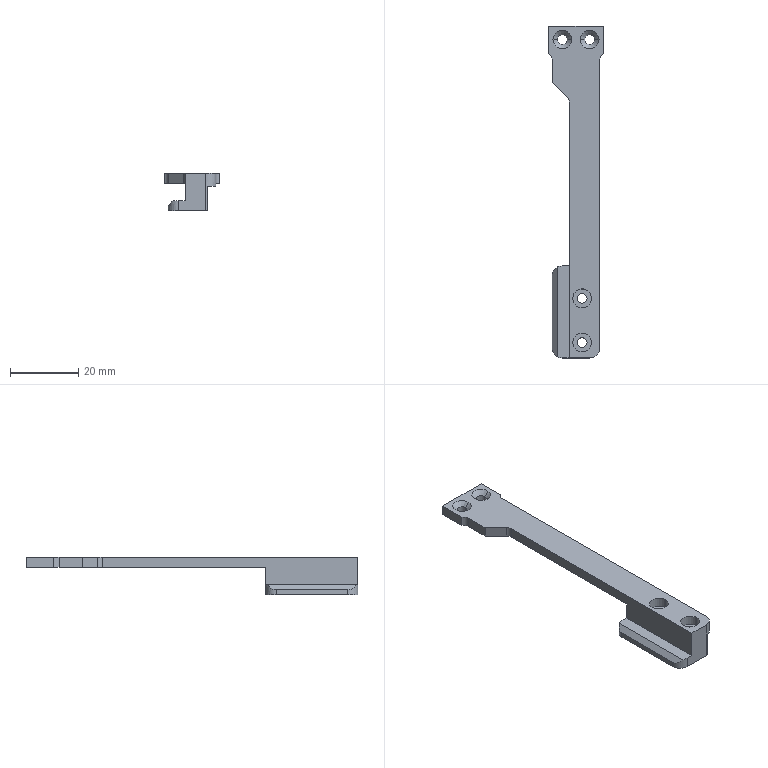NC program | NX | posted with a generic post | part box 16 x 97.4 x 11 mm
Whole program, first 1466 of 1616 lines:
N10 G17 G21 G94 G90
(ADAPTIVE_MILLING_1 , TOOL : D8-25-D8-60-3T-ROUGH)
N12 T02 M6
N14 G54
N16 G17 G0 G90 X-46.305 Y19.064 S6500 M3
N18 G43 Z20. H2
N20 Z-4.9
N22 G94 G1 X-46.303 Y18.914 Z-5.837 F3000.
N24 X-46.3 Y18.764 Z-6.208
N26 X-46.298 Y18.614 Z-6.48
N28 X-46.295 Y18.464 Z-6.7
N30 X-46.293 Y18.314 Z-6.884
N32 X-46.29 Y18.164 Z-7.042
N34 X-46.288 Y18.014 Z-7.18
N36 X-46.286 Y17.864 Z-7.3
N38 X-46.283 Y17.714 Z-7.405
N40 X-46.281 Y17.564 Z-7.498
N42 X-46.278 Y17.414 Z-7.579
N44 X-46.276 Y17.264 Z-7.65
N46 X-46.273 Y17.114 Z-7.71
N48 X-46.271 Y16.964 Z-7.762
N50 X-46.268 Y16.814 Z-7.805
N52 X-46.266 Y16.664 Z-7.839
N54 X-46.263 Y16.514 Z-7.866
N56 X-46.261 Y16.364 Z-7.885
N58 X-46.258 Y16.214 Z-7.896
N60 X-46.256 Y16.064 Z-7.9
N62 X-46.235 Y14.789
N64 G3 X-45.716 Y14.048 R0.809
N66 X-44.438 Y13.739 R5.226
N68 X-41.665 Y13.553 R27.344
N70 X-35.265 Y13.499 R256.654
N72 G1 X49.64
N74 X50.281 Y13.501
N76 X50.921 Y13.487
N78 G2 X53.296 Y12.469 R4.266
N80 X54.935 Y10.214 R6.112
N82 X55.663 Y7.571 R10.548
N84 X55.934 Y4.208 R28.629
N86 X55.996 Y-2.229 R222.094
N88 G1 X55.993 Y-8.303
N90 G2 X55.042 Y-10.705 R4.206
N92 X52.82 Y-12.386 R6.008
N94 X50.123 Y-13.155 R10.335
N96 X46.7 Y-13.435 R28.276
N98 X40.263 Y-13.497 R221.026
N100 G1 X-49.835 Y-13.498
N102 X-50.96 Y-13.483
N104 G2 X-53.325 Y-12.441 R4.293
N106 X-54.923 Y-10.232 R6.094
N108 X-55.667 Y-7.528 R10.64
N110 X-55.933 Y-4.228 R28.613
N112 X-55.996 Y2.209 R217.689
N114 G1 X-56. Y5.266
N116 X-55.992 Y8.324
N118 G2 X-55.066 Y10.671 R4.211
N120 X-52.856 Y12.367 R5.966
N122 X-50.224 Y13.137 R10.16
N124 X-47.3 Y13.377 R16.967
N126 G1 X-46.006 Y13.318
N128 X-44.713 Y13.227
N130 G3 X-38.795 Y13.02 R97.929
N132 G1 X-35.624 Y13.003
N134 X-32.453 Y12.999
N136 X48.734
N138 G2 X52.851 Y11.189 R5.658
N140 X54.443 Y8.596 R7.718
N142 X55.173 Y5.564 R13.413
N144 X55.442 Y1.637 R37.942
N146 X55.492 Y-6.425 R312.321
N148 X53.773 Y-10.266 R5.637
N150 X51.201 Y-11.901 R7.615
N152 X48.177 Y-12.657 R13.076
N154 X44.376 Y-12.936 R35.501
N156 X37.752 Y-12.997 R250.241
N158 G1 X35.002 Y-12.998
N160 X-48.853 Y-12.996
N162 G2 X-52.846 Y-11.19 R5.661
N164 X-54.445 Y-8.582 R7.749
N166 X-55.173 Y-5.551 R13.49
N168 X-55.438 Y-1.749 R37.037
N170 X-55.496 Y5.126 R274.031
N172 G1 X-55.5 Y5.875
N174 X-55.481 Y6.625
N176 G2 X-53.801 Y10.236 R5.633
N178 X-51.157 Y11.916 R7.618
N180 X-47.871 Y12.628 R11.221
N182 X-44.748 Y12.667 R30.947
N184 G3 X-33.138 Y12.501 R329.166
N186 G1 X-29.641 Y12.499
N188 X46.922
N190 G2 X49.208 Y12.216 R7.846
N192 X52.557 Y9.903 R6.635
N194 X54.044 Y7.031 R9.19
N196 X54.713 Y3.726 R16.717
N198 X54.947 Y-0.328 R47.28
N200 X54.983 Y-4.953 R131.72
N202 X52.578 Y-9.913 R6.579
N204 X49.608 Y-11.519 R9.017
N206 X46.309 Y-12.204 R16.357
N208 X42.318 Y-12.444 R45.46
N210 X34.755 Y-12.497 R345.421
N212 G1 X-46.132 Y-12.498
N214 X-47.819 Y-12.466
N216 G2 X-52.408 Y-10.084 R6.561
N218 X-54.009 Y-7.135 R8.99
N220 X-54.706 Y-3.774 R16.39
N222 X-54.945 Y0.28 R46.219
N224 G1 X-54.981 Y2.561
N226 X-54.986 Y4.842
N228 G2 X-54.068 Y8.178 R6.681
N230 X-51.185 Y10.832 R7.188
N232 X-48.101 Y11.819 R10.315
N234 X-44.864 Y12.076 R22.321
N236 G1 X-43.864 Y12.085
N238 X-27.664
N240 G3 X-22.382 Y12.005 R137.915
N242 G1 X-18.516 Y11.999
N244 X45.309
N246 G2 X47.427 Y11.86 R12.199
N248 X51.964 Y9.081 R7.185
N250 X53.51 Y6.019 R9.94
N252 X54.187 Y2.652 R17.79
N254 X54.442 Y-1.651 R48.718
N256 X54.447 Y-3.963 R31.467
N258 X53.495 Y-7.299 R7.389
N260 X50.775 Y-10.007 R7.645
N262 X47.652 Y-11.253 R11.295
N264 X44.071 Y-11.792 R22.406
N266 X39.45 Y-11.969 R72.829
N268 G1 X35.669 Y-11.994
N270 X31.888 Y-11.997
N272 X-44.603
N274 G2 X-46.602 Y-11.959 R27.447
N276 X-50.282 Y-10.698 R7.293
N278 X-52.732 Y-7.883 R7.956
N280 X-53.869 Y-4.648 R12.187
N282 X-54.34 Y-0.868 R26.01
N284 X-54.46 Y3.629 R66.215
N286 X-53.891 Y6.494 R7.865
N288 X-51.028 Y9.807 R7.178
N290 X-47.967 Y11.035 R10.032
N292 X-44.749 Y11.463 R19.383
N294 X-40.001 Y11.574 R90.869
N296 G1 X-33.376 Y11.584
N298 X-30.43 Y11.587
N300 X-27.484 Y11.579
N302 G3 X-18.952 Y11.501 R345.09
N304 G1 X-16.204 Y11.5
N306 X43.871
N308 G2 X46.117 Y11.392 R17.117
N310 X51.451 Y8.231 R7.693
N312 X53.002 Y5.033 R10.645
N314 X53.682 Y1.541 R19.181
N316 X53.907 Y-2.513 R36.968
N318 X53.443 Y-5.337 R8.745
N320 X50.631 Y-9.009 R7.665
N322 X47.419 Y-10.533 R10.754
N324 X43.861 Y-11.201 R19.666
N326 X39.494 Y-11.444 R54.318
N328 X31.557 Y-11.497 R385.627
N330 G1 X30.182
N332 X-43.041
N334 G2 X-45.415 Y-11.459 R38.148
N336 X-48.492 Y-10.706 R8.396
N338 X-51.113 Y-8.66 R7.694
N340 G1 X-51.369 Y-8.359
N342 X-51.597 Y-8.036
N344 G2 X-53.07 Y-4.809 R11.035
N346 X-53.713 Y-1.246 R20.386
N348 X-53.906 Y2.56 R36.428
N350 X-53.423 Y5.38 R8.597
N352 X-51.336 Y8.39 R7.279
N354 X-50.295 Y9.478 R11.092
N356 G1 X-49.274 Y10.193
N358 X-48.144 Y10.719
N360 X-46.94 Y11.041
N362 X-45.7 Y11.15
N364 X-24.699
N366 G3 X-20.606 Y11.02 R66.565
N368 G1 X-17.374 Y11.003
N370 X-14.141 Y11.
N372 X42.559
N374 G2 X45.055 Y10.896 R21.521
N376 X48.627 Y9.662 R8.332
N378 X51.431 Y6.654 R8.583
N380 X52.72 Y3.274 R12.664
N382 X53.306 Y-1.682 R23.115
N384 X52.76 Y-4.804 R8.748
N386 X49.991 Y-8.364 R7.928
N388 X46.743 Y-9.949 R10.964
N390 X43.069 Y-10.67 R19.839
N392 X38.453 Y-10.939 R54.157
N394 X30.516 Y-10.996 R368.029
N396 G1 X-22.68 Y-10.997
N398 G3 X-23.46 Y-11.041 R3.21
N400 G1 X-24.701 Y-11.15
N402 X-45.701
N404 X-46.943 Y-11.041
N406 X-48.147 Y-10.718
N408 X-49.276 Y-10.191
N410 X-50.297 Y-9.476
N412 X-51.178 Y-8.595
N414 X-51.893 Y-7.574
N416 X-52.419 Y-6.444
N418 X-52.741 Y-5.24
N420 G2 X-53.283 Y0.049 R143.418
N422 X-53.035 Y3.961 R12.001
N424 G1 X-52.78 Y4.797
N426 X-52.741 Y5.243
N428 X-52.418 Y6.447
N430 X-51.891 Y7.576
N432 X-51.246 Y8.498
N434 G3 X-52.247 Y9.678 R0.8
N436 G1 X-52.451 Y9.545 Z-7.885
N438 X-52.641 Y9.393 Z-7.869
N440 X-53.503 Y8.717 Z-7.8
N442 X-54.402 Y8.012 F15000.
N444 G3 X-54.685 Y7.576 R0.808
N446 G1 X-55.007 Y6.299
N448 X-55.312 Y5.017
N450 G3 X-55.708 Y1.761 R18.608
N452 G1 X-55.863 Y-3.024
N454 G3 X-55.683 Y-3.556 R0.806
N456 G1 X-54.789 Y-4.653
N458 X-54.152 Y-5.426 Z-7.863 F3000.
N460 G3 X-53.641 Y-5.672 Z-7.9 R0.801
N462 X-52.78 Y-4.804 R0.8
N464 G1 X-52.85 Y-3.999
N466 Y4.001
N468 X-52.779 Y4.81
N470 G3 X-53.012 Y5.448 R0.802
N472 G1 X-53.247 Y5.681
N474 X-54.37 Y6.796 Z-7.8
N476 G2 X-54.689 Y7.369 R0.887 F15000.
N478 X-54.559 Y7.893 R0.807
N480 G1 X-52.913 Y10.362
N482 G2 X-51.228 Y11.971 R5.479
N484 X-49.816 Y12.657 R7.452
N486 X-47.934 Y13.222 R12.236
N488 X-45.983 Y13.437 R12.22
N490 X-42.036 Y13.56 R84.088
N492 G1 X-27.092 Y13.656
N494 G2 X-26.429 Y13.312 R0.802
N496 G1 X-26.31 Y13.14
N498 X-25.41 Y11.838 Z-7.9 F3000.
N500 X-25.254 Y11.611
N502 X-25.089 Y11.39
N504 G3 X-24.575 Y11.139 R0.806
N506 G1 X-23.457 Y11.041
N508 G3 X-20.1 Y10.593 R13.649
N510 X-11.516 Y10.5 R239.739
N512 G1 X41.684 Y10.499
N514 G2 X45.592 Y10.12 R15.22
N516 X51.095 Y5.539 R8.644
N518 X52.607 Y-1.982 R15.053
N520 X48.383 Y-8.371 R8.14
N522 X43.296 Y-10.009 R14.576
N524 X36.378 Y-10.458 R52.796
N526 X27.691 Y-10.496 R660.518
N528 G1 X-21.583 Y-10.498
N530 G3 X-22.256 Y-10.719 R1.464
N532 G1 X-23.403 Y-11.026
N534 G3 X-23.833 Y-11.316 R0.808
N536 G1 X-24.25 Y-11.865
N538 X-25.206 Y-13.126 Z-7.8
N540 G2 X-25.798 Y-13.534 R0.886 F15000.
N542 G1 X-25.92 Y-13.544
N544 X-46.688
N546 G2 X-49.702 Y-12.778 R6.536
N548 G1 X-50.044 Y-12.585
N550 X-50.377 Y-12.376
N552 X-52.02 Y-11.268
N554 G2 X-53.343 Y-9.871 R4.439
N556 X-54.449 Y-7.781 R20.2
N558 X-54.909 Y-6.279 R7.49
N560 X-55.563 Y-1.885 R46.393
N562 X-55.504 Y3.02 R19.609
N564 G1 X-55.31 Y4.44
N566 X-55.102 Y5.858
N568 G2 X-53.8 Y9.132 R9.034
N570 G1 X-53.443 Y9.685
N572 X-53.078 Y10.232
N574 G2 X-51.318 Y11.875 R6.623
N576 X-49.37 Y12.813 R9.364
N578 X-46.503 Y13.52 R16.251
N580 X-45.032 Y13.634 R12.935
N582 G1 X-24.694 Y13.979
N584 G2 X-23.899 Y13.352 R0.8
N586 G1 X-23.839 Y13.08
N588 X-23.497 Y11.535 Z-7.9 F3000.
N590 G3 X-22.914 Y10.895 R0.804
N592 G1 X-21.411 Y10.452
N594 G3 X-17.104 Y10.06 R24.39
N596 X-8.953 Y10. R461.545
N598 G1 X40.497 Y9.999
N600 G2 X44.537 Y9.671 R18.213
N602 X50.574 Y4.798 R8.931
N604 X51.9 Y-1.366 R12.155
N606 X47.893 Y-7.674 R8.103
N608 X42.598 Y-9.472 R14.422
N610 X35.37 Y-9.957 R52.872
N612 X26.12 Y-9.996 R677.713
N614 G1 X-19.96 Y-9.997
N616 G3 X-20.964 Y-10.097 R2.886
N618 G1 X-21.919 Y-10.562
N620 G3 X-22.345 Y-11.048 R0.803
N622 G1 X-22.467 Y-11.439
N624 X-22.941 Y-12.948 Z-7.8
N626 G2 X-23.202 Y-13.432 R0.972 F15000.
N628 X-23.699 Y-13.646 R0.807
N630 G1 X-27.811 Y-13.897
N632 X-31.924 Y-14.131
N634 G2 X-42.441 Y-13.875 R77.782
N636 G1 X-47.365 Y-13.42
N638 G2 X-49.982 Y-12.631 R7.102
N640 X-50.987 Y-12.013 R8.643
N642 G1 X-51.549 Y-11.611
N644 X-52.102 Y-11.197
N646 G2 X-53.85 Y-9.092 R7.418
N648 X-54.848 Y-6.533 R10.673
N650 X-55.5 Y-3.642 R39.775
N652 X-55.614 Y-1.681 R8.461
N654 G1 X-55.207 Y5.23
N656 G2 X-54.627 Y7.498 R6.215
N658 X-53.85 Y8.866 R8.818
N660 G1 X-52.812 Y10.347
N662 G2 X-52.046 Y11.203 R5.737
N664 G1 X-51.854 Y11.357
N666 X-51.656 Y11.502
N668 X-51.071 Y11.893
N670 X-50.478 Y12.274
N672 G2 X-48.149 Y13.179 R7.708
N674 X-45.216 Y13.504 R15.237
N676 G1 X-23.977 Y13.775
N678 G2 X-23.197 Y13.195 R0.8
N680 G1 X-23.146 Y13.013
N682 X-22.712 Y11.492 Z-7.9 F3000.
N684 X-22.652 Y11.279
N686 X-22.579 Y11.07
N688 G3 X-22.197 Y10.692 R0.807
N690 X-18.86 Y9.763 R8.541
N692 X-11.565 Y9.508 R77.946
N694 G1 X-6.953 Y9.501
N696 X39.497 Y9.499
N698 G2 X43.786 Y9.155 R19.531
N700 X50.097 Y3.988 R9.196
N702 X51.053 Y-1.474 R9.498
N704 X47.268 Y-7.053 R8.029
N706 X42.064 Y-8.91 R14.124
N708 X35.153 Y-9.44 R47.679
N710 X24.84 Y-9.496 R685.121
N712 G1 X-18.582 Y-9.498
N714 G3 X-20.271 Y-9.629 R7.598
N716 X-21.095 Y-10.171 R5.028
N718 X-21.435 Y-10.861 R0.801
N720 G1 X-21.262 Y-12.434 Z-7.8
N722 X-21.239 Y-12.644 F15000.
N724 X-21.227 Y-12.855
N726 G2 X-22.016 Y-13.61 R0.8
N728 G1 X-43.772 Y-13.861
N730 G2 X-48.086 Y-13.278 R14.904
N732 X-51.156 Y-11.714 R9.781
N734 G1 X-51.943 Y-11.118
N736 X-52.724 Y-10.514
N738 X-53.006 Y-10.276
N740 X-53.277 Y-10.024
N742 G2 X-53.71 Y-9.434 R2.98
N744 X-54.447 Y-7.93 R11.151
N746 X-55.146 Y-5.267 R14.703
N748 X-55.278 Y-3.798 R12.377
N750 G1 X-55.44 Y2.203
N752 G2 X-54.849 Y6.916 R15.719
N754 G1 X-54.675 Y7.533
N756 X-54.488 Y8.145
N758 G2 X-53.144 Y10.276 R5.71
N760 X-51.595 Y11.647 R11.819
N762 X-49.512 Y12.742 R7.979
N764 X-47.421 Y13.313 R11.302
N766 X-46.168 Y13.429 R10.126
N768 X-37.272 Y13.575 R312.239
N770 G1 X-25.967 Y13.581
N772 G2 X-24.11 Y13.493 R20.526
N774 G1 X-23.184 Y13.405
N776 G2 X-22.499 Y12.857 R0.801
N778 G1 X-22.007 Y11.353 Z-7.9 F3000.
N780 X-21.899 Y11.013
N782 X-21.775 Y10.678
N784 G3 X-21.404 Y10.322 R0.808
N786 X-20.449 Y9.841 R23.478
N788 X-16.974 Y9.204 R13.12
N790 X-9.382 Y9.006 R111.302
N792 G1 X-5.016 Y9.001
N794 X38.309 Y9.
N796 G2 X42.73 Y8.71 R23.559
N798 X50.265 Y0.302 R9.178
N800 X47.195 Y-6.022 R7.56
N802 X42.185 Y-8.213 R12.5
N804 X35.605 Y-8.9 R36.911
N806 X24.168 Y-8.996 R404.381
N808 G1 X-16.97
N810 G3 X-19.6 Y-9.151 R13.964
N812 X-20.105 Y-9.478 R1.054
N814 G1 X-20.464 Y-9.729
N816 G3 X-20.802 Y-10.446 R0.801
N818 G1 X-20.792 Y-10.58
N820 X-20.67 Y-12.158 Z-7.8
N822 G2 X-20.716 Y-12.675 R1.011 F15000.
N824 X-21.385 Y-13.168 R0.801
N826 G1 X-23.451 Y-13.352
N828 X-25.518 Y-13.522
N830 G2 X-30.253 Y-13.665 R61.669
N832 G1 X-45.584 Y-13.533
N834 G2 X-49.302 Y-12.883 R11.335
N836 X-51.182 Y-11.951 R9.638
N838 X-52.122 Y-11.298 R8.244
N840 X-52.988 Y-10.338 R4.901
N842 X-54.222 Y-8.319 R20.738
N844 X-54.773 Y-6.85 R7.392
N846 X-55.528 Y-3.478 R43.944
N848 X-55.673 Y-0.539 R11.383
N850 G1 X-55.204 Y5.261
N852 G2 X-54.264 Y8.362 R7.66
N854 X-49.785 Y12.663 R10.114
N856 X-47.384 Y13.351 R7.726
N858 X-44.43 Y13.526 R25.996
N860 G1 X-21.943 Y13.559
N862 G2 X-21.147 Y12.666 R0.8
N864 G1 X-21.175 Y12.426
N866 X-21.359 Y10.854 Z-7.9 F3000.
N868 G3 X-21.022 Y10.12 R0.801
N870 X-18.496 Y9.049 R5.612
N872 X-13.225 Y8.574 R32.298
N874 X-3.329 Y8.501 R443.883
N876 G1 X37.246 Y8.5
N878 G2 X41.857 Y8.227 R26.64
N880 X48.574 Y3.376 R9.125
N882 X47.062 Y-4.888 R7.016
N884 X42.272 Y-7.472 R11.027
N886 X36.157 Y-8.335 R28.801
N888 X24.659 Y-8.495 R242.942
N890 G1 X-15.351
N892 G3 X-18.78 Y-8.639 R23.511
N894 X-19.545 Y-8.918 R1.61
N896 G1 X-19.987 Y-9.36
N898 G3 X-20.22 Y-9.884 R0.806
N900 G1 X-20.248 Y-10.42
N902 X-20.33 Y-12.001 Z-7.8
N904 G2 X-20.908 Y-12.799 R0.808 F15000.
N906 G1 X-22.238 Y-13.179
N908 G2 X-23.793 Y-13.427 R9.587
N910 G1 X-27.834 Y-13.734
N912 X-31.876 Y-14.023
N914 G2 X-42.521 Y-13.849 R71.443
N916 G1 X-47.446 Y-13.399
N918 G2 X-49.685 Y-12.729 R5.967
N920 X-51.017 Y-11.89 R8.858
N922 G1 X-51.801 Y-11.292
N924 X-52.577 Y-10.684
N926 X-52.857 Y-10.443
N928 X-53.125 Y-10.188
N930 G2 X-53.552 Y-9.593 R3.011
N932 X-54.717 Y-6.993 R14.622
N934 X-55.05 Y-5.459 R8.844
N936 G1 X-55.28 Y-3.622
N938 X-55.494 Y-1.783
N940 G2 X-55.406 Y3.37 R23.638
N942 G1 X-55.284 Y4.351
N944 X-55.145 Y5.329
N946 G2 X-54.436 Y7.669 R10.28
N948 X-53.492 Y9.507 R11.89
N950 X-51.925 Y11.248 R6.735
N952 X-49.848 Y12.557 R13.665
N954 X-48.735 Y13.088 R10.021
N956 X-48.02 Y13.254 R3.368
N958 X-44.829 Y13.526 R36.806
N960 G1 X-44.09 Y13.54
N962 X-26.79 Y13.631
N964 G2 X-23.213 Y13.42 R28.16
N966 G1 X-21.431 Y13.2
N968 G2 X-20.731 Y12.356 R0.8
N970 G1 X-20.739 Y12.222
N972 X-20.838 Y10.643 Z-7.9 F3000.
N974 G3 X-20.82 Y10.197 R1.186
N976 X-20.51 Y9.761 R0.807
N978 X-17.799 Y8.588 R6.045
N980 X-12.344 Y8.082 R33.074
N982 X-2.828 Y8.001 R398.643
N984 G1 X36.247 Y8.
N986 G2 X41.046 Y7.736 R29.411
N988 X46.582 Y4.803 R9.282
N990 X46.574 Y-3.923 R6.511
N992 X42.122 Y-6.742 R9.967
N994 X36.289 Y-7.767 R23.955
N996 X27.043 Y-7.99 R143.085
N998 G1 X22.231 Y-7.995
N1000 X-14.719 Y-7.996
N1002 G3 X-18.294 Y-8.179 R22.526
N1004 X-19.2 Y-8.563 R1.558
N1006 X-19.302 Y-9.265 R0.802
N1008 G1 X-19.252 Y-9.419
N1010 X-18.762 Y-10.924 Z-7.8
N1012 G2 X-18.659 Y-11.391 R1.333 F15000.
N1014 X-19.2 Y-12.123 R0.801
N1016 G1 X-20.366 Y-12.525
N1018 X-21.536 Y-12.913
N1020 G2 X-24.914 Y-13.457 R12.999
N1022 X-31.832 Y-13.577 R267.609
N1024 G1 X-45.787 Y-13.624
N1026 G2 X-49.391 Y-12.935 R9.6
N1028 X-51.343 Y-11.904 R8.067
N1030 X-52.525 Y-10.84 R9.768
N1032 X-53.98 Y-8.867 R8.328
N1034 X-54.835 Y-6.774 R9.887
N1036 X-55.044 Y-5.614 R7.91
N1038 G1 X-55.636 Y0.287
N1040 G2 X-55.471 Y4.2 R13.827
N1042 X-53.986 Y8.664 R14.774
N1044 X-52.718 Y10.415 R9.474
N1046 X-51.42 Y11.617 R9.301
N1048 X-50.417 Y12.236 R7.368
N1050 X-48.819 Y12.948 R11.429
N1052 X-47.192 Y13.344 R9.224
N1054 X-44.247 Y13.575 R21.928
N1056 G1 X-25.104 Y13.776
N1058 G2 X-22.361 Y13.353 R8.536
N1060 G1 X-21.025 Y12.915
N1062 G2 X-20.475 Y12.205 R0.801
N1064 G1 X-20.468 Y12.092
N1066 X-20.369 Y10.513 Z-7.9 F3000.
N1068 X-20.351 Y10.195
N1070 X-20.32 Y9.877
N1072 G3 X-20.103 Y9.476 R0.814
N1074 X-18.296 Y8.424 R4.02
N1076 X-13.944 Y7.71 R18.688
N1078 X-5.26 Y7.505 R138.606
N1080 G1 X-1.141 Y7.501
N1082 X35.184
N1084 G2 X40.049 Y7.277 R34.755
N1086 X44.892 Y5.254 R9.571
N1088 X45.883 Y-2.999 R5.985
N1090 X41.736 Y-6.038 R9.034
N1092 X36.059 Y-7.211 R20.853
N1094 X27.253 Y-7.486 R112.741
N1096 G1 X21.066 Y-7.495
N1098 X-13.841 Y-7.496
N1100 G3 X-17.656 Y-7.683 R26.495
N1102 X-18.851 Y-8.105 R2.625
N1104 X-19.224 Y-8.597 R6.533
N1106 G1 X-19.577 Y-8.95
N1108 G3 X-19.774 Y-9.76 R0.801
N1110 G1 X-19.128 Y-11.204 Z-7.8
N1112 G2 X-18.971 Y-11.65 R1.452 F15000.
N1114 X-19.577 Y-12.511 R0.8
N1116 G1 X-20.856 Y-12.824
N1118 X-22.137 Y-13.124
N1120 G2 X-25.39 Y-13.546 R21.019
N1122 G1 X-37.244 Y-14.145
N1124 G2 X-45.107 Y-13.758 R39.527
N1126 G1 X-46.537 Y-13.546
N1128 X-47.966 Y-13.319
N1130 G2 X-50.995 Y-12.174 R9.363
N1132 X-52.654 Y-10.753 R7.079
N1134 X-53.675 Y-9.427 R10.481
N1136 X-54.995 Y-6.151 R10.707
N1138 X-55.16 Y-4.982 R9.43
N1140 G1 X-55.598 Y0.936
N1142 G2 X-55.346 Y4.846 R14.219
N1144 G1 X-55.058 Y6.199
N1146 G2 X-53.518 Y9.362 R9.128
N1148 G1 X-53.106 Y9.916
N1150 X-52.683 Y10.462
N1152 G2 X-50.894 Y11.985 R7.54
N1154 X-47.24 Y13.408 R10.85
N1156 X-46.066 Y13.536 R9.123
N1158 G1 X-26.315 Y14.308
N1160 G2 X-22.578 Y13.54 R7.967
N1162 G1 X-20.804 Y12.694
N1164 G2 X-20.351 Y12.042 R0.802
N1166 G1 X-20.188 Y10.468 Z-7.9 F3000.
N1168 X-20.112 Y9.738
N1170 G3 X-19.882 Y9.255 R0.807
N1172 X-17.794 Y7.979 R4.417
N1174 X-13.251 Y7.224 R19.503
N1176 X-3.699 Y7.004 R147.219
N1178 G1 X-0.953 Y7.002
N1180 X34.247 Y7.001
N1182 G2 X39.3 Y6.779 R37.483
N1184 X43.487 Y5.248 R9.4
N1186 X45.02 Y-2.037 R5.47
N1188 X41.252 Y-5.304 R8.085
N1190 X35.936 Y-6.625 R17.55
N1192 X27.822 Y-6.975 R82.824
N1194 G1 X20.259 Y-6.994
N1196 X-12.719 Y-6.995
N1198 G3 X-17.054 Y-7.19 R31.774
N1200 X-18.526 Y-7.661 R3.673
N1202 X-18.982 Y-8.252 R3.018
N1204 X-19.112 Y-8.868 R0.804
N1206 G1 X-19.02 Y-9.327
N1208 X-18.711 Y-10.879 Z-7.8
N1210 G2 X-18.699 Y-11.399 R0.993 F15000.
N1212 X-18.982 Y-11.813 R0.809
N1214 G1 X-19.374 Y-12.112
N1216 X-19.786 Y-12.382
N1218 X-20.231 Y-12.593
N1220 X-20.69 Y-12.772
N1222 G2 X-22.592 Y-13.26 R8.241
N1224 X-26.029 Y-13.547 R27.836
N1226 G1 X-43.334 Y-13.877
N1228 G2 X-48.872 Y-12.975 R15.476
N1230 X-50.741 Y-12.098 R12.64
N1232 G1 X-51.425 Y-11.71
N1234 X-52.101 Y-11.308
N1236 G2 X-53.259 Y-10.059 R3.584
N1238 G1 X-53.725 Y-9.22
N1240 X-54.177 Y-8.374
N1242 G2 X-55.087 Y-5.06 R9.147
N1244 X-55.282 Y-1.118 R68.32
N1246 G1 X-55.383 Y3.995
N1248 G2 X-54.739 Y7.487 R8.85
N1250 X-53.566 Y9.592 R7.867
N1252 X-51.463 Y11.589 R12.283
N1254 X-48.684 Y13.055 R11.084
N1256 X-46.567 Y13.495 R9.704
N1258 G1 X-46.075 Y13.532
N1260 X-45.582 Y13.551
N1262 X-30.315 Y13.767
N1264 G2 X-23.882 Y13.477 R56.564
N1266 X-21.116 Y12.906 R16.231
N1268 G1 X-19.485 Y12.418
N1270 G2 X-18.977 Y11.34 R0.8
N1272 G1 X-19.043 Y11.183
N1274 X-19.659 Y9.726 Z-7.9 F3000.
N1276 G3 X-19.485 Y8.857 R0.801
N1278 X-17.253 Y7.51 R4.708
N1280 X-12.445 Y6.725 R20.888
N1282 X-3.384 Y6.506 R142.862
N1284 G1 X0.734 Y6.502
N1286 X33.184 Y6.501
N1288 G2 X38.427 Y6.3 R42.926
N1290 X42.03 Y5.149 R8.836
N1292 X43.839 Y-1.228 R4.992
N1294 X40.344 Y-4.677 R7.351
N1296 X35.305 Y-6.074 R15.569
N1298 X27.631 Y-6.467 R69.067
N1300 G1 X19.256 Y-6.494
N1302 X-11.967 Y-6.495
N1304 G3 X-16.656 Y-6.723 R32.45
N1306 X-18.225 Y-7.219 R4.486
N1308 X-18.472 Y-7.498 R2.296
N1310 X-18.418 Y-8.265 R0.801
N1312 G1 X-17.468 Y-9.53 Z-7.8
N1314 X-17.342 Y-9.697 F15000.
N1316 X-17.226 Y-9.871
N1318 G2 X-17.551 Y-10.937 R0.8
N1320 G1 X-19.019 Y-11.753
N1322 X-20.496 Y-12.556
N1324 G2 X-23.899 Y-13.471 R9.239
N1326 G1 X-26.795 Y-13.692
N1328 X-29.692 Y-13.896
N1330 G2 X-39.192 Y-13.904 R82.473
N1332 G1 X-46.103 Y-13.511
N1334 G2 X-48.992 Y-12.961 R11.233
N1336 X-50.191 Y-12.515 R9.738
N1338 X-52.64 Y-10.585 R7.039
N1340 G1 X-53.077 Y-10.049
N1342 X-53.505 Y-9.506
N1344 G2 X-54.896 Y-6.285 R8.209
N1346 G1 X-55.102 Y-5.257
N1348 X-55.297 Y-4.226
N1350 G2 X-55.508 Y0.057 R18.669
N1352 G1 X-55.207 Y4.59
N1354 G2 X-54.138 Y8.568 R10.511
N1356 X-52.054 Y11.074 R7.468
N1358 G1 X-51.472 Y11.524
N1360 X-50.883 Y11.964
N1362 G2 X-49.047 Y12.882 R7.866
N1364 X-45.683 Y13.502 R10.775
N1366 G1 X-29.672 Y13.864
N1368 G2 X-24.14 Y13.546 R34.768
N1370 G1 X-23.159 Y13.414
N1372 X-22.18 Y13.265
N1374 G2 X-20.304 Y12.66 R7.963
N1376 G1 X-19.222 Y12.155
N1378 G2 X-18.79 Y11.214 R0.8
N1380 G1 X-18.84 Y11.035
N1382 X-19.269 Y9.512 Z-7.9 F3000.
N1384 X-19.36 Y9.155
N1386 G3 X-19.222 Y8.595 R0.806
N1388 X-17.748 Y7.424 R3.271
N1390 X-13.691 Y6.416 R13.773
N1392 X-5.977 Y6.031 R73.953
N1394 G1 X2.234 Y6.002
N1396 X32.996 Y6.
N1398 G2 X37.986 Y5.761 R36.379
N1400 X40.892 Y4.696 R6.252
N1402 X42.345 Y-0.536 R4.561
N1404 X39.202 Y-4.059 R6.699
N1406 X34.39 Y-5.536 R13.767
N1408 X27.532 Y-5.954 R56.808
N1410 X18.345 Y-5.994 R676.366
N1412 G1 X-10.968 Y-5.995
N1414 G3 X-15.972 Y-6.207 R39.83
N1416 X-18.032 Y-6.836 R5.183
N1418 X-18.509 Y-7.576 R1.66
N1420 G1 X-18.688 Y-7.832
N1422 G3 X-18.816 Y-8.452 R0.804
N1424 G1 X-18.703 Y-9.003
N1426 X-18.386 Y-10.553 Z-7.8
N1428 G2 X-18.688 Y-11.392 R0.803 F15000.
N1430 G1 X-19.244 Y-11.803
N1432 X-19.808 Y-12.203
N1434 G2 X-23.12 Y-13.314 R7.079
N1436 X-33.973 Y-13.901 R177.112
N1438 X-41.379 Y-13.776 R98.284
N1440 G1 X-46.318 Y-13.505
N1442 G2 X-51.704 Y-11.391 R9.332
N1444 X-52.931 Y-10.258 R9.375
N1446 X-53.943 Y-8.806 R9.494
N1448 X-54.692 Y-7.202 R9.345
N1450 X-54.982 Y-6.06 R7.658
N1452 G1 X-55.203 Y-4.763
N1454 X-55.412 Y-3.464
N1456 G2 X-55.52 Y1.763 R22.228
N1458 G1 X-55.134 Y5.702
N1460 G2 X-53.613 Y9.256 R6.528
N1462 G1 X-53.001 Y9.983
N1464 X-52.377 Y10.701
N1466 G2 X-50.399 Y12.22 R7.825
N1468 X-48.523 Y13.077 R10.898
N1470 X-46.208 Y13.487 R7.837
N1472 G1 X-28.929 Y13.898
N1474 G2 X-23.975 Y13.548 R26.419
N1476 G1 X-23.2 Y13.42
N1478 X-22.429 Y13.279
N1480 G2 X-20.278 Y12.519 R9.182
N1482 G1 X-19.043 Y11.899
N1484 G2 X-18.629 Y10.976 R0.8
N1486 G1 X-18.66 Y10.863
N1488 X-19.071 Y9.335 Z-7.9 F3000.
N1490 X-19.182 Y8.891
N1492 G3 X-19.043 Y8.339 R0.806
N1494 X-17.38 Y6.987 R3.617
N1496 X-13.351 Y5.958 R14.007
N1498 X-5.718 Y5.539 R69.589
N1500 G1 X2.484 Y5.502
N1502 X32.184 Y5.5
N1504 G2 X37.051 Y5.286 R37.701
N1506 X40.585 Y0.619 R4.009
N1508 X38.091 Y-3.206 R5.789
N1510 X33.752 Y-4.905 R10.938
N1512 X27.531 Y-5.429 R39.85
N1514 X17.532 Y-5.494 R582.791
N1516 G1 X-10.341 Y-5.495
N1518 G3 X-15.656 Y-5.741 R39.498
N1520 X-17.833 Y-6.433 R5.509
N1522 X-18.308 Y-7.146 R1.522
N1524 X-18.273 Y-7.889 R0.802
N1526 G1 X-18.182 Y-8.045
N1528 X-17.382 Y-9.41 Z-7.8
N1530 X-17.205 Y-9.733 F15000.
N1532 G2 X-17.387 Y-10.585 R0.801
N1534 G1 X-17.735 Y-10.934
N1536 X-18.106 Y-11.259
N1538 X-18.307 Y-11.4
N1540 X-18.514 Y-11.532
N1542 X-19.325 Y-12.004
N1544 X-20.143 Y-12.464
N1546 G2 X-23.536 Y-13.381 R8.136
N1548 X-31.437 Y-13.649 R292.441
N1550 G1 X-43.305 Y-13.869
N1552 G2 X-47.708 Y-13.426 R19.484
N1554 X-52.678 Y-10.502 R8.718
N1556 X-53.905 Y-8.838 R10.972
N1558 X-55.059 Y-5.711 R10.078
N1560 G1 X-55.143 Y-5.226
N1562 X-55.211 Y-4.737
N1564 X-55.418 Y-2.938
N1566 X-55.609 Y-1.137
N1568 G2 X-55.385 Y4.085 R20.992
N1570 G1 X-55.228 Y5.024
N1572 X-55.056 Y5.961
N1574 G2 X-54.166 Y8.302 R8.59
N1576 X-53.043 Y10.035 R11.129
N1578 X-50.692 Y12.109 R9.208
N1580 X-49.632 Y12.621 R7.31
N1582 X-47.562 Y13.261 R11.682
N1584 X-46.315 Y13.426 R10.536
N1586 X-40.393 Y13.726 R130.864
N1588 G1 X-37.366 Y13.81
N1590 X-34.339 Y13.879
N1592 G2 X-26.347 Y13.652 R97.006
N1594 G1 X-23.359 Y13.443
N1596 G2 X-20.259 Y12.459 R6.913
N1598 G1 X-18.828 Y11.592
N1600 G2 X-18.474 Y10.68 R0.803
N1602 G1 X-18.84 Y9.141 Z-7.9 F3000.
N1604 X-18.913 Y8.843
N1606 X-18.971 Y8.542
N1608 G3 X-18.828 Y8.032 R0.807
N1610 X-16.94 Y6.505 R3.953
N1612 X-12.57 Y5.44 R15.413
N1614 X-4.538 Y5.034 R77.863
N1616 G1 X3.921 Y5.002
N1618 X31.246 Y5.001
N1620 G2 X35.367 Y4.873 R39.435
N1622 X38.123 Y1.666 R3.407
N1624 X36.394 Y-2.325 R4.994
N1626 X32.39 Y-4.296 R8.873
N1628 X26.807 Y-4.905 R28.919
N1630 X15.995 Y-4.993 R385.603
N1632 G1 X-9.343 Y-4.994
N1634 G3 X-14.944 Y-5.216 R48.215
N1636 X-17.422 Y-5.888 R7.37
N1638 X-17.976 Y-6.425 R1.109
N1640 X-17.92 Y-6.979 R0.806
N1642 G1 X-17.694 Y-7.44
N1644 X-16.996 Y-8.86 Z-7.8
N1646 G2 X-16.873 Y-9.507 R0.918 F15000.
N1648 X-17.055 Y-9.864 R0.832
N1650 G1 X-17.511 Y-10.383
N1652 X-17.977 Y-10.893
N1654 G2 X-19.2 Y-11.873 R6.922
N1656 G1 X-19.758 Y-12.225
N1658 X-20.321 Y-12.567
N1660 G2 X-21.837 Y-13.138 R5.698
N1662 X-23.784 Y-13.392 R11.458
N1664 X-33.169 Y-13.729 R440.822
N1666 G1 X-40.587 Y-13.905
N1668 G2 X-46.487 Y-13.54 R34.749
N1670 G1 X-47.429 Y-13.403
N1672 X-48.367 Y-13.251
N1674 G2 X-50.705 Y-12.361 R7.736
N1676 X-51.676 Y-11.752 R8.786
N1678 X-52.616 Y-10.852 R5.591
N1680 X-53.719 Y-9.221 R10.457
N1682 X-54.628 Y-7.247 R11.413
N1684 X-54.949 Y-6.031 R10.205
N1686 X-55.459 Y-1.921 R28.626
N1688 G1 X-55.474 Y-1.032
N1690 X-55.454 Y-0.144
N1692 X-55.203 Y5.289
N1694 G2 X-53.876 Y8.922 R6.526
N1696 G1 X-52.779 Y10.362
N1698 G2 X-51.866 Y11.306 R6.276
N1700 X-49.926 Y12.538 R12.45
N1702 X-47.118 Y13.407 R8.861
N1704 X-45.647 Y13.532 R12.905
N1706 G1 X-29.603 Y13.924
N1708 G2 X-23.038 Y13.383 R32.012
N1710 X-19.547 Y12.128 R12.594
N1712 G1 X-17.655 Y11.112
N1714 G2 X-17.438 Y9.874 R0.8
N1716 G1 X-17.567 Y9.73
N1718 X-18.567 Y8.605 Z-7.895 F3000.
N1720 X-18.609 Y8.541 Z-7.9
N1722 G3 X-18.577 Y7.673 R0.801
N1724 X-17.006 Y6.255 R3.51
N1726 X-12.953 Y5.076 R13.206
N1728 X-5.384 Y4.561 R60.026
N1730 X4.172 Y4.503 R656.944
N1732 G1 X30.434 Y4.501
N1734 G2 X32.557 Y4.456 R22.366
N1736 X34.618 Y2.411 R2.72
N1738 X33.578 Y-1.546 R4.336
N1740 X29.918 Y-3.723 R7.465
N1742 X25.037 Y-4.386 R21.57
N1744 X14.413 Y-4.493 R281.131
N1746 G1 X-8.655 Y-4.494
N1748 G3 X-14.518 Y-4.728 R50.858
N1750 X-17.189 Y-5.443 R8.134
N1752 X-17.982 Y-6.447 R1.3
N1754 G1 X-18.14 Y-6.786
N1756 G3 X-18.106 Y-7.529 R0.802
N1758 G1 X-17.976 Y-7.75
N1760 X-17.176 Y-9.116 Z-7.8
N1762 G2 X-16.985 Y-9.63 R1.043 F15000.
N1764 X-17.219 Y-10.225 R0.803
N1766 G1 X-17.684 Y-10.691
N1768 X-18.155 Y-11.15
N1770 G2 X-19.5 Y-12.07 R6.218
N1772 G1 X-20.253 Y-12.451
N1774 X-21.012 Y-12.822
N1776 G2 X-24.851 Y-13.642 R9.401
N1778 G1 X-46.348
N1780 G2 X-50.033 Y-12.475 R6.513
N1782 G1 X-51.251 Y-11.634
N1784 X-52.46 Y-10.781
N1786 X-52.751 Y-10.555
N1788 X-53.03 Y-10.312
N1790 G2 X-53.47 Y-9.73 R2.659
N1792 X-54.655 Y-7.035 R12.672
N1794 X-55.266 Y-4.158 R12.831
N1796 G1 X-55.638 Y-0.217
N1798 G2 X-55.373 Y4.666 R16.567
N1800 G1 X-55.187 Y5.586
N1802 X-54.985 Y6.503
N1804 G2 X-54.171 Y8.389 R7.455
N1806 X-53.332 Y9.603 R11.135
N1808 G1 X-52.903 Y10.143
N1810 X-52.463 Y10.675
N1812 G2 X-50.889 Y12.001 R7.69
N1814 X-48.487 Y13.123 R9.525
N1816 X-45.763 Y13.528 R11.208
N1818 G1 X-31.232 Y13.941
N1820 G2 X-24.733 Y13.613 R41.346
N1822 G1 X-23.991 Y13.516
N1824 X-23.25 Y13.41
N1826 G2 X-19.528 Y12.074 R11.552
N1828 G1 X-17.56 Y10.956
N1830 G2 X-17.314 Y9.781 R0.8
N1832 G1 X-17.463 Y9.582
N1834 X-18.411 Y8.314 Z-7.9 F3000.
N1836 G3 X-18.481 Y7.517 R0.801
N1838 X-17.178 Y6.084 R2.997
N1840 X-13.531 Y4.774 R10.928
N1842 X-6.645 Y4.115 R44.208
N1844 X4.359 Y4.003 R367.921
N1846 G1 X28.028 Y4.002
N1848 G2 X29.017 Y3.514 R1.639
N1850 X29.846 Y-0.627 R3.665
N1852 X26.467 Y-3.451 R4.979
N1854 X23.124 Y-3.87 R16.439
N1856 X13.563 Y-3.992 R210.859
N1858 G1 X-6.664 Y-3.993
N1860 G3 X-13.592 Y-4.181 R75.762
N1862 X-16.839 Y-4.933 R10.181
N1864 X-17.76 Y-5.67 R1.886
N1866 G1 X-17.896 Y-6.129
N1868 G3 X-17.657 Y-6.932 R0.801
N1870 X-17.023 Y-7.133 Z-7.857 R0.842
N1872 G1 X-16.126 Y-7.104 Z-7.8
N1874 X-14.458 Y-7.05 F15000.
N1876 X14.716
N1878 G3 X21.591 Y-6.476 R41.519
N1880 G1 X24.029 Y-6.067
N1882 G3 X26.328 Y-4.935 R4.577
N1884 X27.177 Y-3.952 R5.214
N1886 X27.978 Y-2.582 R9.095
N1888 X28.3 Y2.053 R6.69
N1890 X27.818 Y3.335 R6.128
N1892 X25.945 Y5.228 R4.718
N1894 X22.258 Y6.313 R8.152
N1896 G1 X-14.91 Y8.1
N1898 X-16.615 Y8.238
N1900 X-17.599 Y8.312 Z-7.862 F3000.
N1902 G3 X-18.14 Y8.103 Z-7.9 R0.801
N1904 X-18.323 Y7.177 R0.801
N1906 X-16.937 Y5.66 R3.196
N1908 X-13.049 Y4.279 R11.535
N1910 X-9.174 Y3.791 R34.607
N1912 G2 X-4.424 Y3.831 R307.031
N1914 G1 X15.201 Y3.833
N1916 G3 X21.394 Y3.903 R226.847
N1918 G1 X21.642 Y3.988
N1920 G3 X21.908 Y5.34 Z-7.8 R0.883
N1922 X21.293 Y5.648 R0.884 F15000.
N1924 G1 X-16.529 Y8.038
N1926 X-16.986 Y8.07 Z-7.829 F3000.
N1928 X-17.444 Y8.086 Z-7.858
N1930 G3 X-18.025 Y7.793 Z-7.9 R0.901
N1932 X-18.164 Y6.837 R0.881
N1934 X-16.799 Y5.296 R3.261
N1936 X-12.939 Y3.855 R11.322
N1938 X-11.65 Y3.66 R5.855
N1940 G1 X-11.521 Y3.687
N1942 G3 X-10.997 Y4.961 Z-7.8 R0.883
N1944 X-11.419 Y5.341 R0.887 F15000.
N1946 G1 X-16.236 Y7.405
N1948 X-16.606 Y7.566 Z-7.826 F3000.
N1950 X-16.981 Y7.714 Z-7.851
N1952 G3 X-17.719 Y7.577 Z-7.9 R0.892
N1954 X-18.006 Y6.497 R0.88
N1956 X-16.841 Y5.048 R2.972
N1958 X-13.77 Y3.658 R9.902
N1960 G2 X-12.721 Y2.086 R2.48
N1962 X-13.31 Y-1.021 R4.054
N1964 X-15.737 Y-3.452 R8.695
N1966 G3 X-17.481 Y-4.866 R10.565
N1968 X-17.652 Y-5.197 R2.627
N1970 X-17.272 Y-6.017 R0.801
N1972 X-16.528 Y-6.06 Z-7.851 R0.83
N1974 G1 X-15.765 Y-5.792 Z-7.8
N1976 X-14.926 Y-5.501 F15000.
N1978 X-14.092 Y-5.197
N1980 X-13.761 Y-5.032
N1982 X-13.437 Y-4.856
N1984 G3 X-12.882 Y-4.383 R2.604
N1986 G1 X-10.787 Y-1.986
N1988 G3 X-10.136 Y-0.252 R2.636
N1990 X-10.504 Y1.654 R5.133
N1992 G1 X-10.747 Y2.257
N1994 X-10.998 Y2.857
N1996 G3 X-12.772 Y5.471 R9.518
N1998 G1 X-14.526 Y7.305
N2000 G3 X-15.166 Y7.55 R0.802
N2002 G1 X-16.256 Y7.466
N2004 X-17.311 Y7.38 Z-7.867 F3000.
N2006 G3 X-17.769 Y7.145 Z-7.9 R0.804
N2008 X-17.965 Y6.384 R0.801
N2010 X-16.92 Y4.834 R2.744
N2012 G2 X-15.571 Y3.45 R4.509
N2014 X-15.352 Y-0.425 R4.731
N2016 X-16.907 Y-3.183 R10.833
N2018 G3 X-17.57 Y-4.302 R4.477
N2020 G1 X-17.659 Y-5.243
N2022 X-17.805 Y-5.786
N2024 G3 X-17.249 Y-6.763 R0.8
N2026 X-16.511 Y-6.605 Z-7.85 R0.829
N2028 G1 X-15.859 Y-6.144 Z-7.8
N2030 X-15.134 Y-5.631 F15000.
N2032 G3 X-14.796 Y-4.98 R0.802
N2034 G1 X-14.769 Y6.082
N2036 G3 X-15.463 Y6.877 R0.8
N2038 G1 X-16.052 Y6.955
N2040 X-17.068 Y7.085 Z-7.865 F3000.
N2042 G3 X-17.591 Y6.929 Z-7.9 R0.802
N2044 X-17.884 Y6.082 R0.801
N2046 X-17.257 Y4.866 R2.811
N2048 G2 X-16.452 Y0.023 R5.936
N2050 X-17.496 Y-2.843 R19.278
N2052 G1 X-17.55 Y-3.086
N2054 G2 X-17.583 Y-4.374 R12.617
N2056 G3 X-16.659 Y-5.234 R0.8
N2058 X-16.088 Y-4.844 Z-7.855 R0.843
N2060 G1 X-15.585 Y-4.136 Z-7.8
N2062 X-14.563 Y-2.7 F15000.
N2064 X-14.5 Y-2.594
N2066 X-14.102 Y-1.805
N2068 X-13.718 Y-1.009
N2070 G3 X-13.53 Y1.499 R4.022
N2072 G1 X-14.364 Y4.859
N2074 G3 X-14.682 Y5.322 R0.806
N2076 G1 X-15.837 Y6.129
N2078 X-16.231 Y6.407 Z-7.831 F3000.
N2080 X-16.631 Y6.677 Z-7.861
N2082 G3 X-17.226 Y6.763 Z-7.9 R0.8
N2084 X-17.803 Y5.78 R0.8
N2086 G2 X-17.198 Y3.541 R25.873
N2088 X-17.526 Y-0.91 R10.214
N2090 G1 X-17.55 Y-1.058
N2092 Y-3.12
N2094 G3 X-16.769 Y-3.92 R0.8
N2096 X-16.088 Y-3.576 Z-7.85 R0.833
N2098 G1 X-15.579 Y-2.973 Z-7.8
N2100 X-14.655 Y-1.881 F15000.
N2102 G3 X-14.467 Y-1.34 R0.806
N2104 G1 X-14.623 Y3.638
N2106 G3 X-14.783 Y4.093 R0.811
N2108 G1 X-15.668 Y5.272
N2110 X-15.999 Y5.717 Z-7.835 F3000.
N2112 X-16.338 Y6.155 Z-7.87
N2114 G3 X-16.734 Y6.4 Z-7.9 R0.804
N2116 X-17.706 Y5.418 R0.8
N2118 G1 X-17.659 Y5.24
N2120 X-17.55 Y3.999
N2122 Y-1.063
N2124 G3 X-16.618 Y-1.862 R0.808
N2126 G1 X-15.572 Y-1.699
N2128 X-15.424 Y-1.676 Z-7.896
N2130 X-15.276 Y-1.653 Z-7.885
N2132 X-15.127 Y-1.63 Z-7.866
N2134 X-14.979 Y-1.607 Z-7.839
N2136 X-14.831 Y-1.584 Z-7.805
N2138 X-14.683 Y-1.561 Z-7.762
N2140 X-14.535 Y-1.538 Z-7.71
N2142 X-14.386 Y-1.515 Z-7.65
N2144 X-14.238 Y-1.492 Z-7.579
N2146 X-14.09 Y-1.469 Z-7.498
N2148 X-13.942 Y-1.446 Z-7.405
N2150 X-13.793 Y-1.423 Z-7.3
N2152 X-13.645 Y-1.4 Z-7.18
N2154 X-13.497 Y-1.377 Z-7.042
N2156 X-13.349 Y-1.354 Z-6.884
N2158 X-13.201 Y-1.331 Z-6.7
N2160 X-13.052 Y-1.308 Z-6.48
N2162 X-12.904 Y-1.285 Z-6.208
N2164 X-12.756 Y-1.261 Z-5.837
N2166 X-12.608 Y-1.238 Z-4.9
N2168 G0 Z20.
N2170 X-57.731 Y5.189
N2172 Z-3.908
N2174 G1 X-57.581 Y5.193 Z-4.845
N2176 X-57.431 Y5.198 Z-5.216
N2178 X-57.281 Y5.202 Z-5.489
N2180 X-57.131 Y5.207 Z-5.708
N2182 X-56.982 Y5.211 Z-5.893
N2184 X-56.832 Y5.216 Z-6.051
N2186 X-56.682 Y5.22 Z-6.188
N2188 X-56.532 Y5.225 Z-6.308
N2190 X-56.382 Y5.229 Z-6.414
N2192 X-56.232 Y5.234 Z-6.506
N2194 X-56.082 Y5.238 Z-6.587
N2196 X-55.932 Y5.243 Z-6.658
N2198 X-55.782 Y5.247 Z-6.719
N2200 X-55.632 Y5.252 Z-6.77
N2202 X-55.482 Y5.256 Z-6.813
N2204 X-55.332 Y5.261 Z-6.848
N2206 X-55.182 Y5.265 Z-6.874
N2208 X-55.032 Y5.269 Z-6.893
N2210 X-54.882 Y5.274 Z-6.905
N2212 X-54.733 Y5.278 Z-6.908
N2214 X-53.294 Y5.321
N2216 G3 X-52.542 Y5.902 R0.809
N2218 G1 X-52.478 Y6.121
N2220 X-51.999 Y6.962
N2222 G2 X-49.146 Y9.337 R10.485
N2224 X-45.127 Y10.426 R10.966
N2226 X-38.946 Y10.642 R66.81
N2228 X-25.684 Y10.63 R881.917
N2230 X-20.854 Y8.845 R7.721
N2232 G3 X-20.256 Y8.349 R2.794
N2234 G1 X-19.945 Y8.241
N2236 X-19.159 Y7.749
N2238 X-18.503 Y7.094
N2240 X-18.008 Y6.31
N2242 X-17.82 Y5.78
N2244 G3 X-16.276 Y5.918 R0.8
N2246 G1 X-16.271 Y6.139 Z-6.894
N2248 X-16.296 Y6.36 Z-6.88
N2250 X-16.421 Y7.491 Z-6.808
N2252 X-16.547 Y8.641 F15000.
N2254 G3 X-16.899 Y9.219 R0.802
N2256 G1 X-20.192 Y11.414
N2258 G3 X-23.793 Y12.784 R8.656
N2260 X-27.725 Y13.068 R29.736
N2262 G1 X-39.62 Y13.135
N2264 G3 X-45.48 Y12.79 R45.623
N2266 G1 X-46.413 Y12.675
N2268 X-47.345 Y12.547
N2270 G3 X-49.868 Y11.829 R12.012
N2272 G1 X-51.337 Y11.23
N2274 G3 X-51.791 Y10.75 R0.803
N2276 G1 X-52.236 Y9.462
N2278 X-52.551 Y8.533 Z-6.87 F3000.
N2280 G3 X-52.48 Y7.951 Z-6.908 R0.801
N2282 X-51.337 Y7.67 R0.8
N2284 G2 X-49.334 Y8.721 R7.482
N2286 X-43.303 Y9.977 R19.447
N2288 X-34.306 Y10.147 R146.553
N2290 X-26.724 Y10.122 R356.688
N2292 X-22.321 Y8.869 R9.325
N2294 G3 X-21.741 Y8.65 R1.479
N2296 G1 X-20.821 Y8.546
N2298 X-20.23 Y8.34
N2300 G3 X-19.407 Y9.668 R0.8
N2302 G1 X-19.602 Y9.813 Z-6.893
N2304 X-19.808 Y9.94 Z-6.878
N2306 X-20.738 Y10.522 Z-6.808
N2308 X-21.099 Y10.75 F15000.
N2310 X-21.466 Y10.968
N2312 X-21.624 Y11.019
N2314 X-21.788 Y11.038
N2316 X-49.723 Y11.213
N2318 G3 X-50.372 Y10.888 R0.802
N2320 G1 X-50.888 Y10.189
N2322 X-51.482 Y9.376 Z-6.872 F3000.
N2324 G3 X-51.594 Y8.826 Z-6.908 R0.801
N2326 X-50.529 Y8.204 R0.8
N2328 G1 X-49.62 Y8.537
N2330 G3 X-45.963 Y9.132 R129.918
N2332 G2 X-38.359 Y9.615 R58.221
N2334 X-24.598 Y9.633 R615.66
N2336 X-23.574 Y9.075 R5.367
N2338 G3 X-22.603 Y8.65 R2.669
N2340 G1 X-21.741
N2342 G3 X-20.945 Y9.531 R0.8
N2344 X-21.341 Y10.147 Z-6.86 R0.838
N2346 G1 X-22.014 Y10.621 Z-6.808
N2348 X-22.835 Y11.201 F15000.
N2350 G3 X-23.299 Y11.348 R0.811
N2352 G1 X-47.628 Y11.286
N2354 G3 X-48.07 Y11.151 R0.813
N2356 G1 X-48.861 Y10.623
N2358 X-49.321 Y10.319 Z-6.843 F3000.
N2360 X-49.776 Y10.005 Z-6.878
N2362 G3 X-50.043 Y9.619 Z-6.908 R0.804
N2364 X-49.185 Y8.588 R0.8
N2366 G2 X-47.283 Y8.65 R11.759
N2368 X-41.487 Y9.01 R935.154
N2370 X-26.505 Y9.134 R364.319
N2372 X-24.445 Y8.65 R35.426
N2374 G1 X-22.57
N2376 G3 X-21.774 Y9.532 R0.8
N2378 X-22.17 Y10.147 Z-6.86 R0.838
N2380 G1 X-22.843 Y10.621 Z-6.808
N2382 X-23.666 Y11.202 F15000.
N2384 G3 X-24.127 Y11.348 R0.811
N2386 G1 X-45.725
N2388 G3 X-46.186 Y11.202 R0.811
N2390 G1 X-46.988 Y10.636
N2392 X-47.794 Y10.062 Z-6.871 F3000.
N2394 G3 X-48.076 Y9.557 Z-6.908 R0.801
N2396 X-47.283 Y8.65 R0.8
N2398 G1 X-24.408
N2400 G3 X-23.604 Y9.538 R0.808
N2402 G1 X-23.712 Y10.628
N2404 X-23.727 Y10.777 Z-6.905
N2406 X-23.742 Y10.926 Z-6.893
N2408 X-23.756 Y11.076 Z-6.874
N2410 X-23.771 Y11.225 Z-6.848
N2412 X-23.786 Y11.374 Z-6.813
N2414 X-23.801 Y11.523 Z-6.77
N2416 X-23.815 Y11.673 Z-6.719
N2418 X-23.83 Y11.822 Z-6.658
N2420 X-23.845 Y11.971 Z-6.587
N2422 X-23.86 Y12.121 Z-6.506
N2424 X-23.875 Y12.27 Z-6.414
N2426 X-23.889 Y12.419 Z-6.308
N2428 X-23.904 Y12.568 Z-6.188
N2430 X-23.919 Y12.718 Z-6.051
N2432 X-23.934 Y12.867 Z-5.893
N2434 X-23.949 Y13.016 Z-5.708
N2436 X-23.963 Y13.165 Z-5.489
N2438 X-23.978 Y13.315 Z-5.216
N2440 X-23.993 Y13.464 Z-4.845
N2442 X-24.008 Y13.613 Z-3.908
N2444 G0 Z20.
N2446 X-50.953 Y13.294
N2448 Z3.1
N2450 G1 X-50.893 Y13.157 Z2.163
N2452 X-50.833 Y13.019 Z1.792
N2454 X-50.773 Y12.881 Z1.52
N2456 X-50.714 Y12.744 Z1.3
N2458 X-50.654 Y12.606 Z1.116
N2460 X-50.594 Y12.469 Z0.958
N2462 X-50.534 Y12.331 Z0.82
N2464 X-50.475 Y12.193 Z0.7
N2466 X-50.415 Y12.056 Z0.595
N2468 X-50.355 Y11.918 Z0.502
N2470 X-50.295 Y11.781 Z0.421
N2472 X-50.236 Y11.643 Z0.35
N2474 X-50.176 Y11.506 Z0.29
N2476 X-50.116 Y11.368 Z0.238
N2478 X-50.056 Y11.23 Z0.195
N2480 X-49.997 Y11.093 Z0.161
N2482 X-49.937 Y10.955 Z0.134
N2484 X-49.877 Y10.818 Z0.115
N2486 X-49.817 Y10.68 Z0.104
N2488 X-49.758 Y10.542 Z0.1
N2490 X-49.145 Y9.132
N2492 G3 X-48.694 Y8.7 R0.812
N2494 X-46.19 Y8.274 R8.595
N2496 X-38.242 Y8.151 R151.011
N2498 G1 X-23.618 Y8.15
N2500 G2 X-20.019 Y6.32 R4.504
N2502 X-18.442 Y2.471 R8.427
N2504 X-18.139 Y-3.635 R29.257
N2506 X-21.022 Y-8.897 R7.113
N2508 X-24.98 Y-10.333 R9.009
N2510 X-30.718 Y-10.634 R44.455
N2512 G1 X-44.542 Y-10.635
N2514 G2 X-49.364 Y-8.994 R7.889
N2516 X-51.822 Y-4.81 R7.327
N2518 X-52.298 Y-0.029 R24.53
N2520 X-52.298 Y3.157 R30.584
N2522 X-50.226 Y6.172 R4.471
N2524 X-46.459 Y7.417 R8.812
N2526 X-41.529 Y7.64 R44.369
N2528 G1 X-36.592 Y7.65
N2530 G2 X-24.955 Y7.634 R875.956
N2532 X-20.371 Y4.743 R5.952
N2534 X-18.909 Y0.391 R11.013
N2536 X-18.898 Y-3.838 R12.406
N2538 X-23.036 Y-8.859 R6.957
N2540 X-27.768 Y-9.944 R14.567
N2542 X-35.201 Y-10.145 R96.274
N2544 X-43.643 Y-10.123 R410.756
N2546 X-47.862 Y-8.928 R8.345
N2548 X-50.885 Y-4.861 R7.687
N2550 X-51.711 Y-0.009 R18.345
N2552 X-49.183 Y5.308 R5.534
N2554 X-44.975 Y6.802 R10.098
N2556 X-39.176 Y7.13 R44.035
N2558 X-26.432 Y7.13 R770.628
N2560 X-20.867 Y3.607 R6.788
N2562 X-19.543 Y-2.771 R10.387
N2564 X-23.254 Y-7.906 R7.035
N2566 X-28.085 Y-9.322 R13.305
N2568 X-35.199 Y-9.636 R64.623
N2570 X-42.823 Y-9.61 R207.132
N2572 X-47.084 Y-8.346 R8.33
N2574 X-50.258 Y-4.077 R8.348
N2576 X-50.986 Y-0.227 R11.464
N2578 X-48.134 Y4.652 R6.124
N2580 X-43.691 Y6.243 R10.987
N2582 X-37.458 Y6.625 R45.242
N2584 X-27.696 Y6.625 R382.732
N2586 X-21.24 Y2.357 R7.455
N2588 X-20.493 Y-2.675 R7.584
N2590 X-24.024 Y-7.244 R7.129
N2592 X-28.888 Y-8.759 R13.357
N2594 X-35.312 Y-9.122 R53.861
N2596 X-42.123 Y-9.091 R116.39
N2598 X-47.206 Y-7.099 R8.176
N2600 X-50.034 Y-1.603 R8.767
N2602 X-47.567 Y3.702 R6.133
N2604 X-43.052 Y5.605 R10.465
N2606 X-37.33 Y6.096 R35.136
N2608 X-28.83 Y6.121 R219.961
N2610 X-22.666 Y2.929 R7.815
N2612 X-23.633 Y-5.704 R6.31
N2614 X-28.15 Y-7.903 R10.321
N2616 X-33.854 Y-8.554 R29.735
N2618 X-41.227 Y-8.583 R92.609
N2620 X-46.49 Y-6.54 R8.568
N2622 X-48.833 Y-2.702 R7.057
N2624 X-46.843 Y2.811 R5.914
N2626 X-42.558 Y4.925 R9.753
N2628 X-36.852 Y5.565 R28.853
N2630 X-29.666 Y5.602 R107.37
N2632 X-24.664 Y3.726 R8.28
N2634 X-23.945 Y-4.335 R5.692
N2636 X-28.086 Y-7.054 R8.772
N2638 X-33.307 Y-7.959 R21.218
N2640 X-40.552 Y-8.055 R60.279
N2642 X-45.756 Y-6.012 R8.734
N2644 X-46.484 Y1.307 R5.313
N2646 X-42.47 Y4.069 R8.2
N2648 X-37.251 Y4.976 R20.299
N2650 X-30.318 Y5.067 R60.454
N2652 X-26.152 Y3.703 R8.239
N2654 X-24.678 Y-2.972 R5.077
N2656 X-28.283 Y-6.145 R7.477
N2658 X-33.373 Y-7.358 R16.403
N2660 X-39.864 Y-7.52 R40.606
N2662 X-43.993 Y-6.218 R8.706
N2664 X-45.563 Y-0.065 R4.778
N2666 X-42.108 Y3.152 R7.056
N2668 X-37.278 Y4.353 R15.178
N2670 X-31.037 Y4.528 R38.246
N2672 X-27.817 Y3.622 R7.441
N2674 X-25.965 Y-1.837 R4.531
N2676 X-29.05 Y-5.313 R6.56
N2678 X-33.626 Y-6.726 R13.095
N2680 X-39.67 Y-6.914 R24.823
N2682 X-42.499 Y-5.977 R6.24
N2684 X-44.021 Y-1.079 R4.283
N2686 X-40.956 Y2.419 R6.307
N2688 X-36.427 Y3.772 R12.86
N2690 X-31.255 Y3.908 R20.925
N2692 X-27.789 Y-0.731 R3.95
N2694 X-30.329 Y-4.518 R5.73
N2696 X-34.819 Y-6.162 R10.991
N2698 X-39.051 Y-6.296 R14.343
N2700 X-41.909 Y-2.694 R3.561
N2702 X-39.902 Y1.241 R5.173
N2704 X-35.82 Y3.051 R9.255
N2706 X-33.277 Y3.302 R9.666
N2708 X-30.669 Y0.715 R3.076
N2710 X-31.949 Y-3.247 R4.622
N2712 X-35.31 Y-5.189 R6.618
N2714 X-37.32 Y-4.296 R3.055
N2716 G3 X-37.665 Y-4.112 R1.519
N2718 X-38.217 Y-4.17 Z0.136 R0.864
N2720 G1 X-39.167 Y-4.534 Z0.2
N2722 X-39.56 Y-4.688 F15000.
N2724 X-39.959 Y-4.826
N2726 G2 X-40.88 Y-4.296 R0.8
N2728 G1 X-41.174 Y-3.42
N2730 X-41.455 Y-2.54
N2732 G2 X-41.626 Y-0.011 R6.459
N2734 G1 X-41.542 Y0.655
N2736 X-41.44 Y1.317
N2738 G2 X-39.798 Y3.858 R4.191
N2740 G1 X-38.339 Y4.917
N2742 G2 X-37.351 Y4.879 R0.8
N2744 G1 X-36.797 Y4.407
N2746 X-35.593 Y3.381 Z0.1 F3000.
N2748 X-35.45 Y3.259
N2750 G3 X-34.999 Y3.039 R2.018
N2752 G1 X-34.854 Y2.999 Z0.104
N2754 X-34.71 Y2.96 Z0.115
N2756 X-34.565 Y2.92 Z0.134
N2758 X-34.42 Y2.88 Z0.161
N2760 X-34.276 Y2.841 Z0.195
N2762 X-34.131 Y2.801 Z0.238
N2764 X-33.986 Y2.761 Z0.29
N2766 X-33.842 Y2.722 Z0.35
N2768 X-33.697 Y2.682 Z0.421
N2770 X-33.552 Y2.643 Z0.502
N2772 X-33.408 Y2.603 Z0.595
N2774 X-33.263 Y2.563 Z0.7
N2776 X-33.118 Y2.524 Z0.82
N2778 X-32.974 Y2.484 Z0.958
N2780 X-32.829 Y2.444 Z1.116
N2782 X-32.684 Y2.405 Z1.3
N2784 X-32.54 Y2.365 Z1.52
N2786 X-32.395 Y2.326 Z1.792
N2788 X-32.25 Y2.286 Z2.163
N2790 X-32.106 Y2.246 Z3.1
N2792 G0 Z20.
N2794 M5
(PLANAR_MILL_5_COPY , TOOL : D4-12-D4-50-3T-FINISH)
N2796 T06 M6
N2798 G54
N2800 G17 G0 G90 X-52.658 Y6.5 S6500 M3
N2802 G43 Z20. H6
N2804 Z-5.2
N2806 G94 G1 Z-7.2 F800.
N2808 X-48.658
N2810 X-21.742
N2812 X-17.742
N2814 Z-5.2
N2816 G0 Z20.
(PLANAR_MILL_5_COPY_1 , TOOL : D4-12-D4-50-3T-FINISH)
N2818 X-26.7 Y11.
N2820 Z-6.
N2822 G1 Z-8.
N2824 G3 X-24.7 Y9. R2.
N2826 G2 X-19.7 Y4. R5.
N2828 G1 Y-4.
N2830 G2 X-24.7 Y-9. R5.
N2832 G3 X-26.7 Y-11. R2.
N2834 G1 Z-6.
N2836 G0 Z20.
N2838 M5
(PLANAR_MILL_8 , TOOL : D50面刀)
N2840 T01 M6
N2842 G54
N2844 G17 G0 G90 X5.258 Y-0.5 S4500 M3
N2846 G43 Z20. H1
N2848 Z2.
N2850 G94 G1 Z0. F600.
N2852 X-21.742
N2854 X-48.658
N2856 X-75.658
N2858 Z2.
N2860 G0 Z20.
(PLANAR_MILL_10 , TOOL : D50面刀)
N2862 X33.8 Y42.6
N2864 Z-6.
N2866 G1 Z-8.
N2868 Y7.6
N2870 Y-6.3
N2872 Y-41.3
N2874 Z-6.
N2876 G0 Z20.
N2878 X3.8 Y42.6
N2880 Z-6.
N2882 G1 Z-8.
N2884 Y7.6
N2886 Y-6.3
N2888 Y-41.3
N2890 Z-6.
N2892 G0 Z20.
N2894 M5
(DRILLING_1 , TOOL : 倒角D6-90度)
N2896 T03 M6
N2898 G54
N2900 G17 G0 G90 X-44.2 Y1.799 S3000 M3
N2902 G43 Z20. H3
N2904 G94 G81 G99 Z-1.55 F200. R3.
N2906 X-31.2
N2908 G80
N2910 G0 X-31.2 Y1.799 Z20.
(DRILLING_1_COPY , TOOL : 倒角D6-90度)
N2912 X44.7 Y4.
N2914 G81 Z-9.55 F200. R-5.
N2916 Y-4.
N2918 G80
N2920 G0 X44.7 Y-4. Z20.
(PLANAR_MILL_6 , TOOL : 倒角D6-90度)
N2922 X-51.2 Y3.5 S3500
N2924 Z0.5